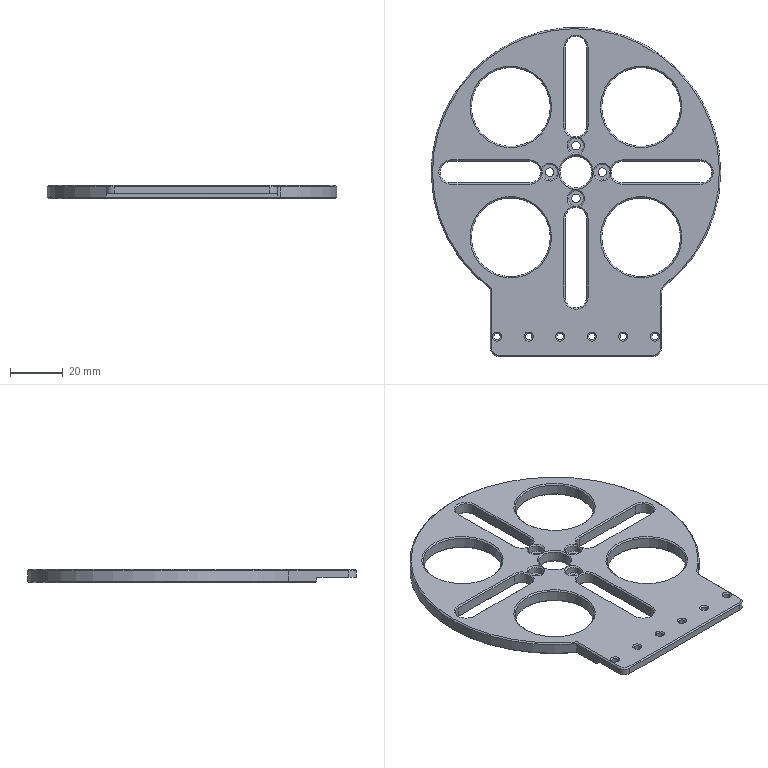Part | NX | 1 solid | 118 faces | box 110 x 125 x 5 mm | volume 30079 mm3 | cone 46 | plane 41 | cylinder 31 | commonest cylinder face diameters 8.2 x8 2.5 x6 3.2 x4 5.8 x4 30 x4 6 x3